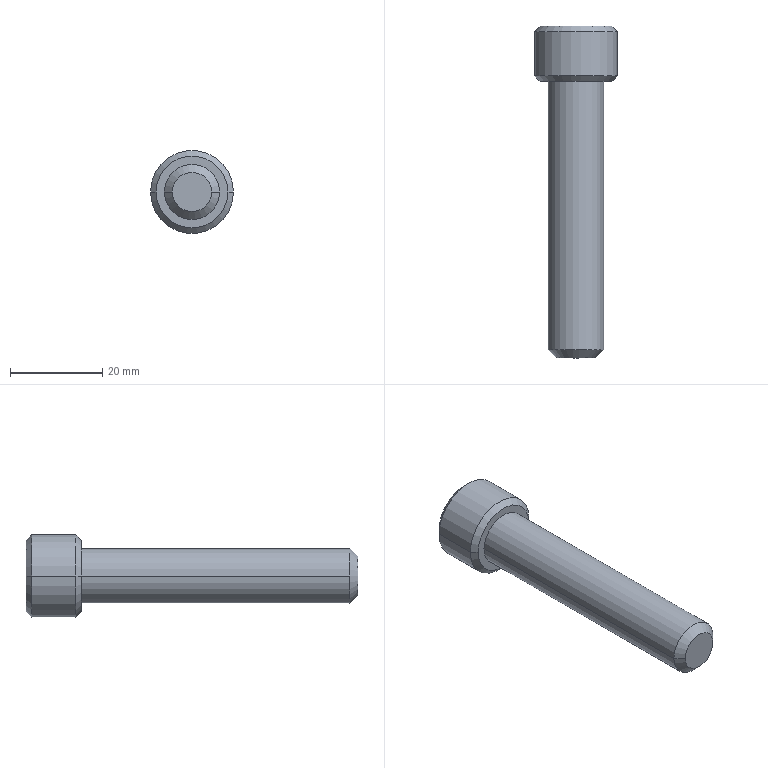Part | STEP file | BB62-M12-60L | 1 solid | 27 faces | box 18 x 72 x 18 mm | volume 9088 mm3 | plane 15 | cone 8 | cylinder 4 | commonest cylinder face diameters 12 x2 18 x2